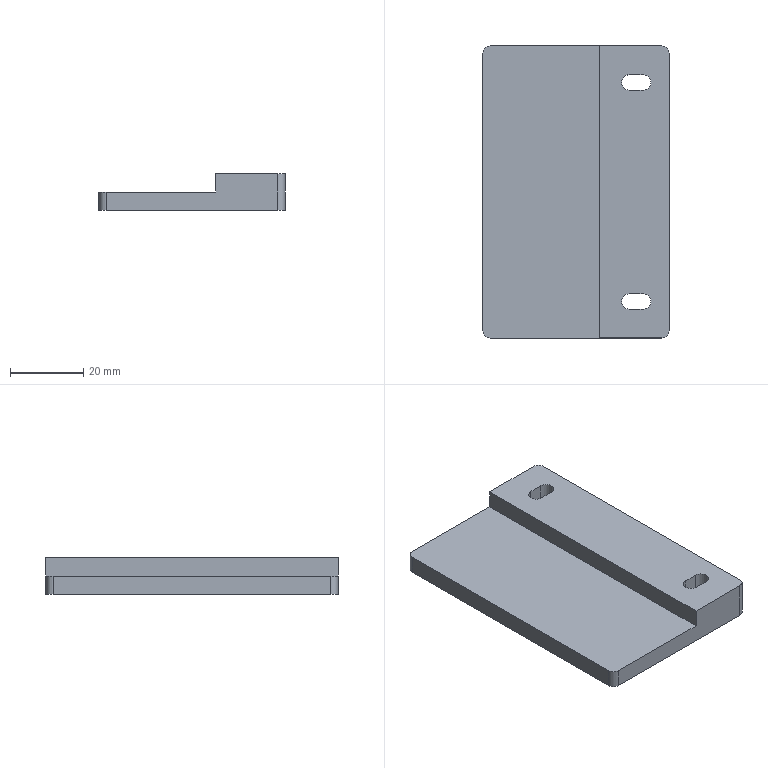Part | STEP file | 1 solid | 22 faces | box 51 x 80 x 10 mm | volume 27378 mm3 | plane 12 | cylinder 10 | commonest cylinder face diameters 4.2 x6 4 x4